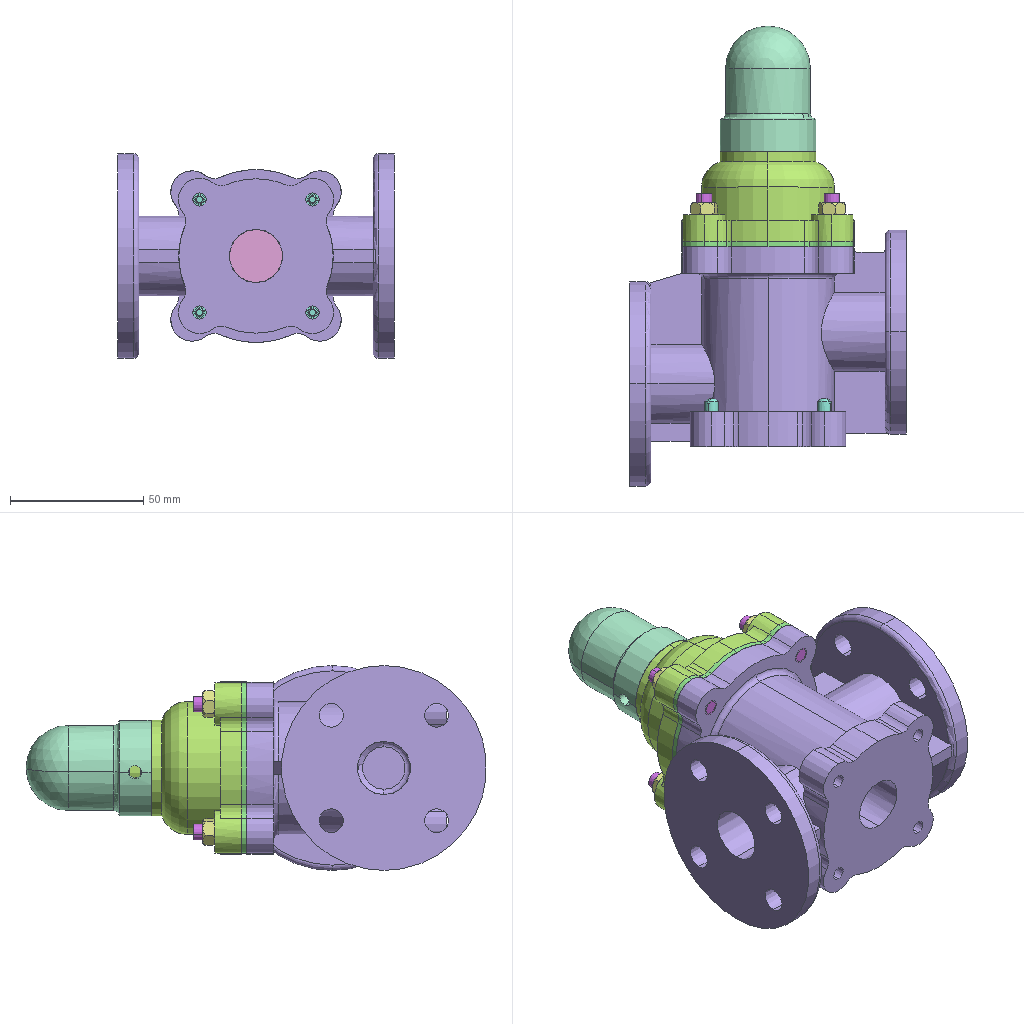Assembly | SolidWorks | 13 different items | 25 placed | box 104 x 173 x 77 mm
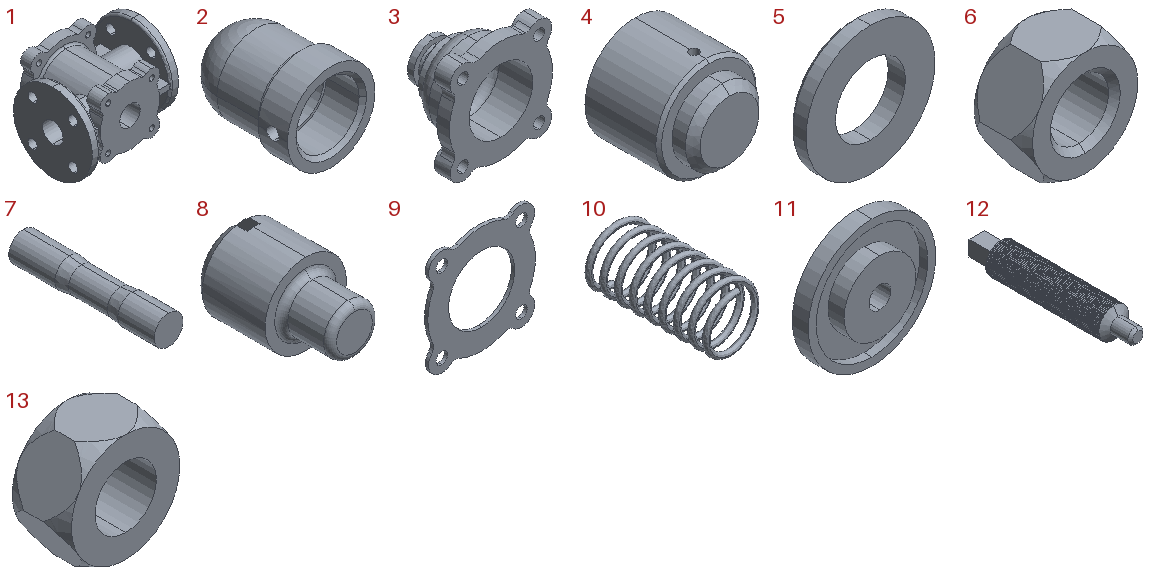Parts list (item | quantity | size | volume | features):
1 | x1 | 104 x 96.5 x 77 mm | 206017 mm3 | features ICE 14, Fillet 9, Rib 4, 3DProfileFeature 2, HoleWzd 2, Chamfer 1, Extrusion 1, RevCut 1
2 | x1 | 36 x 47 x 36 mm | 17147 mm3 | features Chamfer 1, ICE 1, Revolution 1
3 | x1 | 65 x 46 x 65 mm | 47923 mm3 | features ICE 3, Chamfer 1, Fillet 1, HoleWzd 1, Revolution 1
4 | x1 | 34 x 32 x 34 mm | 12156 mm3 | features HoleWzd 1, ICE 1, Revolution 1
5 | x4 | 12 x 1.6 x 12 mm | 124.914 mm3 | features Chamfer 1, Extrusion 1
6 | x4 | 10.392 x 5 x 9 mm | 243.63 mm3 | features ICE 3, Chamfer 2, Extrusion 1
7 | x4 | 6 x 30 x 6 mm | 787.114 mm3 | features Revolution 1
8 | x4 | 5 x 8 x 5 mm | 104.473 mm3 | features Fillet 2, ICE 1, Revolution 1
9 | x1 | 65 x 2 x 65 mm | 4890 mm3 | features Fillet 2, Extrusion 1
10 | x1 | 27.466 x 58.241 x 27.466 mm | 3289 mm3 | features Helix 1, Sweep 1
11 | x1 | 32 x 6 x 32 mm | 2776 mm3 | features Revolution 1
12 | x1 | 10 x 53 x 10 mm | 3177 mm3 | features ICE 1, Revolution 1, SweepThread 1
13 | x1 | 17.321 x 8.2 x 15 mm | 1094 mm3 | features ICE 2, Extrusion 1, HoleWzd 1
Mates (type | each side: item.copy, entity, surface, feature):
Concentric | 4.1 edge | 1.1 edge
Coincident | 4.1 face cone Revolve1 | 1.1 face cone Cut-Revolve1
Coincident | 11.1 face cone Revolve1 | 12.1 face cone Revolve1
Concentric | 12.1 edge | 13.1 edge
Coincident | 1.1 face plane Boss-Extrude1 | 9.1 face plane Boss-Extrude1
Concentric | 4.1 edge | 9.1 edge
Concentric | 10.1 select_type:24 | 4.1 face cylinder Revolve1
Concentric | 11.1 edge | 4.1 edge
Coincident | 3.1 edge | 9.1 edge | 2 times
Coincident | 3.1 face plane Revolve1 | 5.1 face plane Boss-Extrude1
Concentric | 5.1 edge | 6.1 edge
Coincident | 5.1 face plane Boss-Extrude1 | 6.1 face plane Boss-Extrude1
Concentric | 6.1 edge | 7.1 edge
Coincident | 1.1 face plane Boss-Extrude1 | 7.1 face plane Revolve1
Coincident | 3.1 face plane Revolve1 | 13.1 face plane Boss-Extrude1
Coincident | 3.1 face plane Revolve1 | 2.1 face plane Revolve1
Concentric | 3.1 edge | 2.1 edge
Concentric | 3.1 edge | 7.1 edge
Concentric | 1.1 edge | 7.1 edge